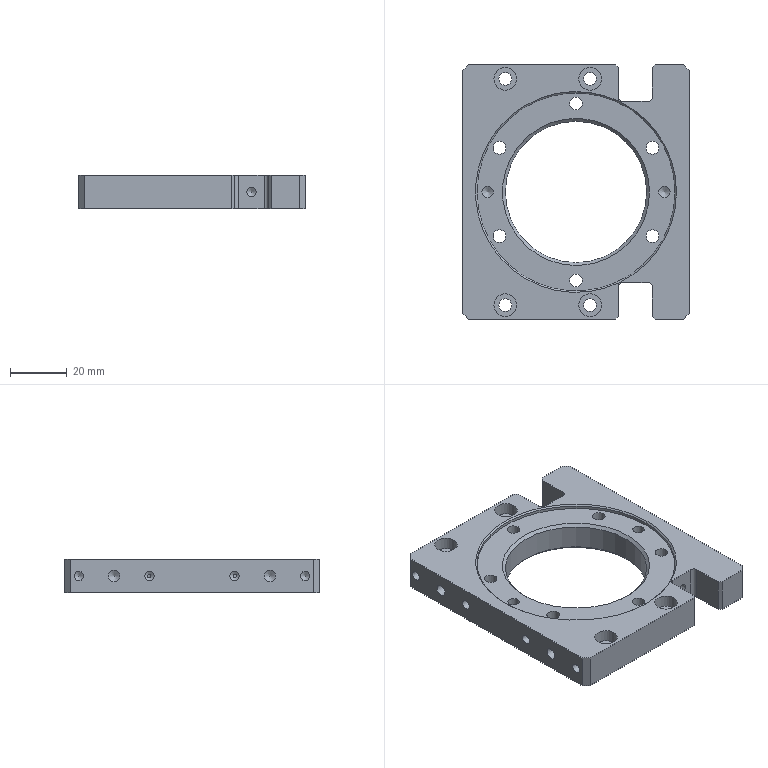CAM job | NX | 3-axis milling, drilling | part box 80 x 90 x 12 mm | stock box 85 x 95 x 15 mm
Tools:
number,name,description,diameter,corner_radius,flute_length,length,flutes
4,D4,平底铣刀-粗,4.0,0.0,25.0,75.0,2
9,D10,平底铣刀-粗,10.0,0.0,35.0,75.0,2
19,D2-J,平底铣刀-精,2.0,0.0,50.0,75.0,2
18,D3-J,平底铣刀-精,3.0,0.0,50.0,75.0,2
7,D6-J,平底铣刀-精,6.0,0.0,25.0,75.0,2
10,D10-J,平底铣刀-精,10.0,0.0,35.0,75.0,2
1,D80R0.8飞刀,圆鼻刀-粗,80.0,0.8,50.0,75.0,2
1,D80R0.8飞刀-J,圆鼻刀-精,80.0,0.8,50.0,75.0,2
2,D6倒角刀,倒角刀,6.0,0.0,3.0,25.0,2
17,ZT3.8,钻头,3.8,0.0,35.0,50.0,2
11,ZT4.5,钻头,4.5,0.0,35.0,50.0,2
Operations:
program,operation,operation_type,tool,method,geometry_group,spindle_rpm,surface_speed,feed_per_tooth,feed_cut,feed_plunge,cut_length_mm,path_length_mm,cut_time_min,machine_time_min
B,底壁铣飞面开粗_COPY,VolumeBased25DMillingOperation,D80R0.8飞刀,分层开粗-切深K-步距G,W-B,2800.0,703.696,0.5357,3000.0,100.0,2320.185,2477.922,0.7734,0.7892
B,底壁铣飞面精光_COPY,VolumeBased25DMillingOperation,D80R0.8飞刀-J,侧刃精光-切深K-步距G,W-B,4000.0,1005.28,0.125,1000.0,100.0,386.11,422.11,0.3861,0.3897
B,铣沉头_1,CylinderMilling,D4,METHOD,W-B,8000.0,100.531,0.1125,1800.0,100.0,1107.396,1528.846,0.6152,0.6574
B,铣孔_1,CylinderMilling,D4,METHOD,W-B,8000.0,100.531,0.0375,600.0,100.0,105.106,555.356,0.1752,0.2202
B,钻倒角_2,Operation,D6倒角刀,METHOD,W-B,8000.0,150.796,0.0625,1000.0,0.0,22.2,233.756,0.0222,0.0434
B,铣倒角_4,PlanarMilling,D6倒角刀,METHOD,W-B,8000.0,150.796,0.0375,600.0,100.0,125.782,541.367,0.2096,0.2512
B,底壁铣倒角_COPY_1,VolumeBased25DMillingOperation,D6倒角刀,爬面_倒角-切深0-步距G,W-B,6500.0,122.519,0.1154,1500.0,100.0,631.295,671.695,0.4209,0.4249
B,C0.3封闭铣廓倒角6X45L_COPY,PlanarMilling,D6倒角刀,爬面_倒角-切深0-步距G,W-B,7000.0,131.0,0.1071,1500.0,100.0,399.82,435.82,0.2665,0.2701
A,顶面,FaceMilling,D80R0.8飞刀,侧刃精光-切深K-步距G,W-A,4000.0,1005.31,0.125,1000.0,100.0,407.333,443.333,0.4073,0.4109
A,外形粗_2,VolumeBased25DMillingOperation,D10,METHOD,W-A,8000.0,251.327,0.3125,5000.0,80.0,6941.916,6992.616,1.388,1.393
A,型腔铣开粗-中_COPY,CavityMilling,D10,分层开粗-切深K-步距G,W-A,8000.0,251.327,0.25,4000.0,100.0,11195.15,11806.208,2.799,2.892
A,打点-深0.8,Operation,D6倒角刀,NONE,W-A,8000.0,150.796,0.0312,500.0,90.0,23.4,352.103,0.0468,0.0797
A,通孔-5-6,Operation,ZT4.5,NONE,W-A,3000.0,42.411,0.025,150.0,90.0,96.0,396.33,0.64,0.67
A,沉头孔-钻孔0段,Operation,ZT4.5,NONE,W-A,2800.0,39.584,0.0179,100.0,90.0,65.408,313.855,0.6541,0.6789
A,盲锥孔-精孔4.0预钻,Operation,ZT3.8,NONE,W-A,3000.0,35.814,0.02,120.0,90.0,14.203,134.915,0.1184,0.1304
A,铣孔开粗D4_1,CylinderMilling,D4,NONE,W-A,8000.0,100.531,0.075,1200.0,100.0,851.827,1167.427,0.7099,0.7414
A,铣孔精光D4_1,CylinderMilling,D4,精光步距切深关,W-A,8000.0,100.531,0.0312,500.0,100.0,128.184,443.784,0.2564,0.2879
A,外形侧面,ZLevelMilling,D3-J,METHOD,W-A,9000.0,84.823,0.1389,2500.0,80.0,2006.065,2221,0.8028,0.8243
A,仅选体,SurfaceContour,D6倒角刀,METHOD,W-A,8000.0,150.796,0.1875,3000.0,100.0,399.67,435.471,0.1332,0.1368
A,钻倒角_1,Operation,D6倒角刀,METHOD,W-A,8000.0,150.796,0.0312,500.0,0.0,10.6,129.772,0.0212,0.0331
A,铣倒角_1,PlanarMilling,D6倒角刀,METHOD,W-A,8000.0,150.796,0.0312,500.0,100.0,104.118,524.961,0.2082,0.2503
A,铣倒角_2,PlanarMilling,D6倒角刀,NONE,W-A,8000.0,150.796,0.0312,500.0,100.0,135.871,421.428,0.2717,0.3003
A,铣倒角_3,PlanarMilling,D6倒角刀,METHOD,W-A,8000.0,150.796,0.0312,500.0,100.0,227.195,268.195,0.4544,0.4585
A,底壁铣倒角_COPY,VolumeBased25DMillingOperation,D6倒角刀,爬面_倒角-切深0-步距G,W-A,6500.0,122.519,0.1154,1500.0,100.0,159.914,203.314,0.1066,0.1109
A,铣孔精光D2_1,CylinderMilling,D2-J,精光步距切深关,W-A,8000.0,50.266,0.0125,200.0,100.0,251.778,409.278,1.259,1.275
A,底壁铣精光侧面-中_COPY,VolumeBased25DMillingOperation,D6-J,侧刃精光-切深K-步距G,W-A,8000.0,150.792,0.0625,1000.0,100.0,289.792,331.668,0.2898,0.294
A,外形半精_2,VolumeBased25DMillingOperation,D6-J,METHOD,W-A,8000.0,251.327,0.0625,1000.0,100.0,403.586,466.986,0.4036,0.4099
A,底壁铣精光侧面-中-选底面_COPY,VolumeBased25DMillingOperation,D10-J,侧刃精光-切深K-步距G,W-A,6000.0,188.496,0.0833,1000.0,100.0,213.842,235.242,0.2138,0.216